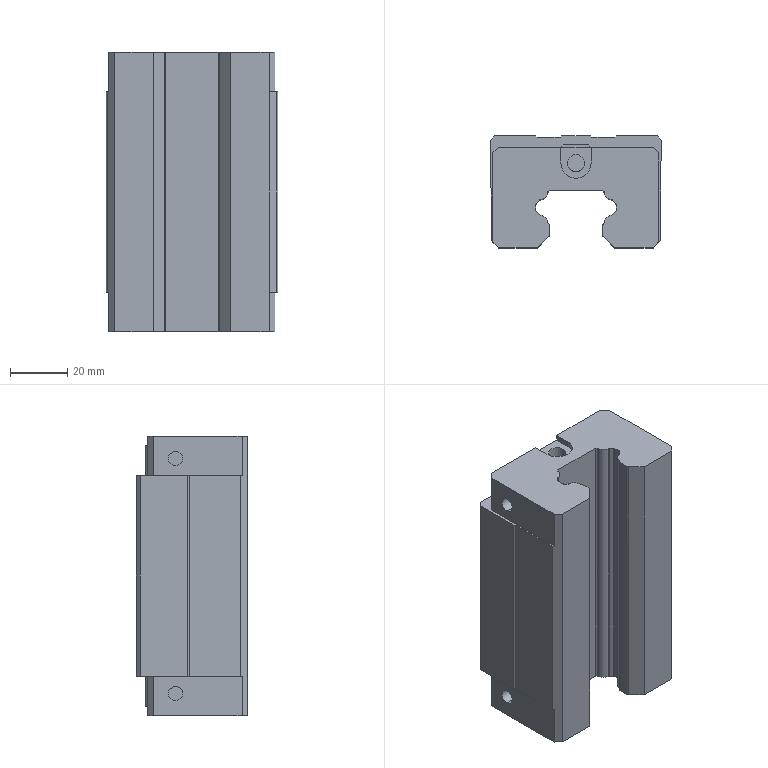Part | SolidWorks | features BaseBody 1 | 1 solid | 140 faces | box 60 x 39.001 x 97.4 mm | volume 169047 mm3 | plane 86 | cylinder 54 | commonest cylinder face diameters 1.2 x12 1 x8 5 x8 8 x8 1.6 x4 5.66 x4